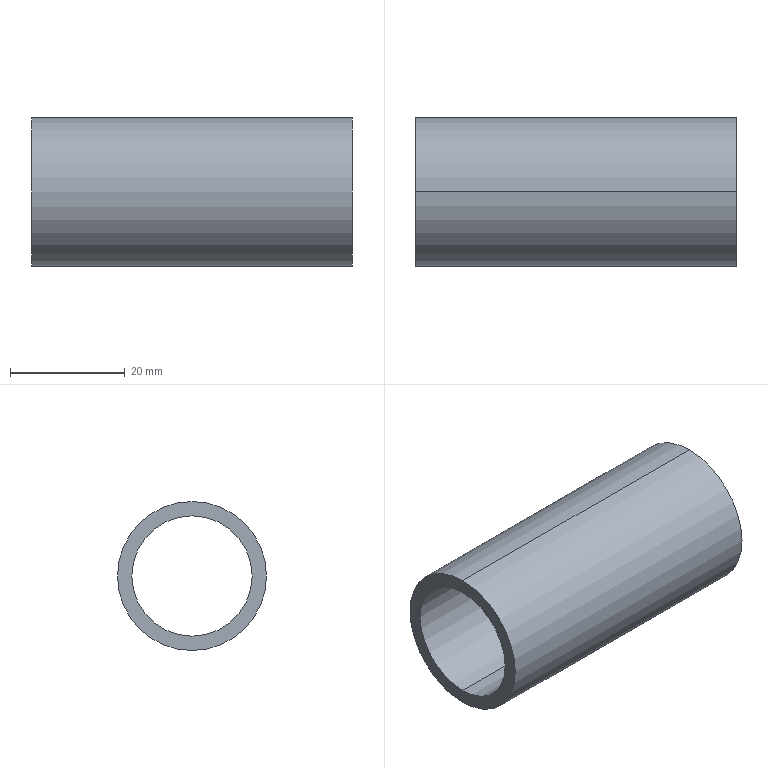Part | SolidWorks | features Extrusion 1 | 1 solid | 6 faces | box 56 x 26 x 26 mm | volume 10336 mm3 | cylinder 4 | plane 2 | commonest cylinder face diameters 21 x2 26 x2
STEP:
#1=CARTESIAN_POINT('',(56.,0.,10.5));
#2=VERTEX_POINT('',#1);
#3=CARTESIAN_POINT('',(56.,0.,-10.5));
#4=VERTEX_POINT('',#3);
#5=CARTESIAN_POINT('',(56.,0.,0.));
#6=DIRECTION('',(1.,0.,0.));
#7=DIRECTION('',(0.,0.,-1.));
#8=AXIS2_PLACEMENT_3D('',#5,#6,#7);
#9=CIRCLE('',#8,10.5);
#10=EDGE_CURVE('',#2,#4,#9,.T.);
#11=ORIENTED_EDGE('',*,*,#10,.T.);
#12=CARTESIAN_POINT('',(0.,0.,-10.5));
#13=VERTEX_POINT('',#12);
#14=CARTESIAN_POINT('',(56.,0.,-10.5));
#15=DIRECTION('',(-1.,0.,0.));
#16=VECTOR('',#15,1000.);
#17=LINE('',#14,#16);
#18=EDGE_CURVE('',#4,#13,#17,.T.);
#19=ORIENTED_EDGE('',*,*,#18,.T.);
#20=CARTESIAN_POINT('',(0.,0.,10.5));
#21=VERTEX_POINT('',#20);
#22=CARTESIAN_POINT('',(0.,0.,0.));
#23=DIRECTION('',(1.,0.,0.));
#24=DIRECTION('',(0.,0.,-1.));
#25=AXIS2_PLACEMENT_3D('',#22,#23,#24);
#26=CIRCLE('',#25,10.5);
#27=EDGE_CURVE('',#21,#13,#26,.T.);
#28=ORIENTED_EDGE('',*,*,#27,.F.);
#29=CARTESIAN_POINT('',(56.,0.,10.5));
#30=DIRECTION('',(-1.,0.,0.));
#31=VECTOR('',#30,1000.);
#32=LINE('',#29,#31);
#33=EDGE_CURVE('',#2,#21,#32,.T.);
#34=ORIENTED_EDGE('',*,*,#33,.F.);
#35=EDGE_LOOP('',(#11,#19,#28,#34));
#36=FACE_OUTER_BOUND('',#35,.T.);
#37=CARTESIAN_POINT('',(56.,0.,0.));
#38=DIRECTION('',(-1.,0.,0.));
#39=DIRECTION('',(0.,0.,1.));
#40=AXIS2_PLACEMENT_3D('',#37,#38,#39);
#41=CYLINDRICAL_SURFACE('',#40,10.5);
#42=ADVANCED_FACE('',(#36),#41,.F.);
#43=CARTESIAN_POINT('',(56.,0.,-13.));
#44=VERTEX_POINT('',#43);
#45=CARTESIAN_POINT('',(56.,0.,13.));
#46=VERTEX_POINT('',#45);
#47=CARTESIAN_POINT('',(56.,0.,0.));
#48=DIRECTION('',(1.,0.,0.));
#49=DIRECTION('',(0.,0.,-1.));
#50=AXIS2_PLACEMENT_3D('',#47,#48,#49);
#51=CIRCLE('',#50,13.);
#52=EDGE_CURVE('',#44,#46,#51,.T.);
#53=ORIENTED_EDGE('',*,*,#52,.F.);
#54=CARTESIAN_POINT('',(0.,0.,-13.));
#55=VERTEX_POINT('',#54);
#56=CARTESIAN_POINT('',(56.,0.,-13.));
#57=DIRECTION('',(-1.,0.,0.));
#58=VECTOR('',#57,1000.);
#59=LINE('',#56,#58);
#60=EDGE_CURVE('',#44,#55,#59,.T.);
#61=ORIENTED_EDGE('',*,*,#60,.T.);
#62=CARTESIAN_POINT('',(0.,0.,13.));
#63=VERTEX_POINT('',#62);
#64=CARTESIAN_POINT('',(0.,0.,0.));
#65=DIRECTION('',(1.,0.,0.));
#66=DIRECTION('',(0.,0.,-1.));
#67=AXIS2_PLACEMENT_3D('',#64,#65,#66);
#68=CIRCLE('',#67,13.);
#69=EDGE_CURVE('',#55,#63,#68,.T.);
#70=ORIENTED_EDGE('',*,*,#69,.T.);
#71=CARTESIAN_POINT('',(56.,0.,13.));
#72=DIRECTION('',(-1.,0.,0.));
#73=VECTOR('',#72,1000.);
#74=LINE('',#71,#73);
#75=EDGE_CURVE('',#46,#63,#74,.T.);
#76=ORIENTED_EDGE('',*,*,#75,.F.);
#77=EDGE_LOOP('',(#53,#61,#70,#76));
#78=FACE_OUTER_BOUND('',#77,.T.);
#79=CARTESIAN_POINT('',(56.,0.,0.));
#80=DIRECTION('',(-1.,0.,0.));
#81=DIRECTION('',(0.,0.,1.));
#82=AXIS2_PLACEMENT_3D('',#79,#80,#81);
#83=CYLINDRICAL_SURFACE('',#82,13.);
#84=ADVANCED_FACE('',(#78),#83,.T.);
#85=CARTESIAN_POINT('',(56.,0.,0.));
#86=DIRECTION('',(1.,0.,0.));
#87=DIRECTION('',(0.,0.,-1.));
#88=AXIS2_PLACEMENT_3D('',#85,#86,#87);
#89=CIRCLE('',#88,13.);
#90=EDGE_CURVE('',#46,#44,#89,.T.);
#91=ORIENTED_EDGE('',*,*,#90,.T.);
#92=ORIENTED_EDGE('',*,*,#52,.T.);
#93=EDGE_LOOP('',(#91,#92));
#94=FACE_OUTER_BOUND('',#93,.T.);
#95=ORIENTED_EDGE('',*,*,#10,.F.);
#96=CARTESIAN_POINT('',(56.,0.,0.));
#97=DIRECTION('',(1.,0.,0.));
#98=DIRECTION('',(0.,0.,-1.));
#99=AXIS2_PLACEMENT_3D('',#96,#97,#98);
#100=CIRCLE('',#99,10.5);
#101=EDGE_CURVE('',#4,#2,#100,.T.);
#102=ORIENTED_EDGE('',*,*,#101,.F.);
#103=EDGE_LOOP('',(#95,#102));
#104=FACE_BOUND('',#103,.T.);
#105=CARTESIAN_POINT('',(56.,0.,0.));
#106=DIRECTION('',(1.,0.,0.));
#107=DIRECTION('',(0.,0.,-1.));
#108=AXIS2_PLACEMENT_3D('',#105,#106,#107);
#109=PLANE('',#108);
#110=ADVANCED_FACE('',(#94,#104),#109,.T.);
#111=CARTESIAN_POINT('',(0.,0.,0.));
#112=DIRECTION('',(1.,0.,0.));
#113=DIRECTION('',(0.,0.,-1.));
#114=AXIS2_PLACEMENT_3D('',#111,#112,#113);
#115=CIRCLE('',#114,13.);
#116=EDGE_CURVE('',#63,#55,#115,.T.);
#117=ORIENTED_EDGE('',*,*,#116,.F.);
#118=ORIENTED_EDGE('',*,*,#69,.F.);
#119=EDGE_LOOP('',(#117,#118));
#120=FACE_OUTER_BOUND('',#119,.T.);
#121=ORIENTED_EDGE('',*,*,#27,.T.);
#122=CARTESIAN_POINT('',(0.,0.,0.));
#123=DIRECTION('',(1.,0.,0.));
#124=DIRECTION('',(0.,0.,-1.));
#125=AXIS2_PLACEMENT_3D('',#122,#123,#124);
#126=CIRCLE('',#125,10.5);
#127=EDGE_CURVE('',#13,#21,#126,.T.);
#128=ORIENTED_EDGE('',*,*,#127,.T.);
#129=EDGE_LOOP('',(#121,#128));
#130=FACE_BOUND('',#129,.T.);
#131=CARTESIAN_POINT('',(0.,0.,0.));
#132=DIRECTION('',(1.,0.,0.));
#133=DIRECTION('',(0.,0.,-1.));
#134=AXIS2_PLACEMENT_3D('',#131,#132,#133);
#135=PLANE('',#134);
#136=ADVANCED_FACE('',(#120,#130),#135,.F.);
#137=ORIENTED_EDGE('',*,*,#60,.F.);
#138=ORIENTED_EDGE('',*,*,#90,.F.);
#139=ORIENTED_EDGE('',*,*,#75,.T.);
#140=ORIENTED_EDGE('',*,*,#116,.T.);
#141=EDGE_LOOP('',(#137,#138,#139,#140));
#142=FACE_OUTER_BOUND('',#141,.T.);
#143=CARTESIAN_POINT('',(56.,0.,0.));
#144=DIRECTION('',(-1.,0.,0.));
#145=DIRECTION('',(0.,0.,1.));
#146=AXIS2_PLACEMENT_3D('',#143,#144,#145);
#147=CYLINDRICAL_SURFACE('',#146,13.);
#148=ADVANCED_FACE('',(#142),#147,.T.);
#149=ORIENTED_EDGE('',*,*,#18,.F.);
#150=ORIENTED_EDGE('',*,*,#101,.T.);
#151=ORIENTED_EDGE('',*,*,#33,.T.);
#152=ORIENTED_EDGE('',*,*,#127,.F.);
#153=EDGE_LOOP('',(#149,#150,#151,#152));
#154=FACE_OUTER_BOUND('',#153,.T.);
#155=CARTESIAN_POINT('',(56.,0.,0.));
#156=DIRECTION('',(-1.,0.,0.));
#157=DIRECTION('',(0.,0.,1.));
#158=AXIS2_PLACEMENT_3D('',#155,#156,#157);
#159=CYLINDRICAL_SURFACE('',#158,10.5);
#160=ADVANCED_FACE('',(#154),#159,.F.);
#161=CLOSED_SHELL('',(#42,#84,#110,#136,#148,#160));
#162=MANIFOLD_SOLID_BREP('',#161);
#163=CARTESIAN_POINT('',(0.,0.,0.));
#164=DIRECTION('',(0.,0.,1.));
#165=DIRECTION('',(1.,0.,0.));
#166=AXIS2_PLACEMENT_3D('',#163,#164,#165);
#167=(LENGTH_UNIT()NAMED_UNIT(*)SI_UNIT(.MILLI.,.METRE.));
#168=UNCERTAINTY_MEASURE_WITH_UNIT(LENGTH_MEASURE(0.00001),#167,'','');
#169=(NAMED_UNIT(*)PLANE_ANGLE_UNIT()SI_UNIT($,.RADIAN.));
#170=(NAMED_UNIT(*)SI_UNIT($,.STERADIAN.)SOLID_ANGLE_UNIT());
#171=(GEOMETRIC_REPRESENTATION_CONTEXT(3)GLOBAL_UNCERTAINTY_ASSIGNED_CONTEXT((#168))GLOBAL_UNIT_ASSIGNED_CONTEXT((#167,#169,#170))REPRESENTATION_CONTEXT('',''));
#172=ADVANCED_BREP_SHAPE_REPRESENTATION('',(#162,#166),#171);